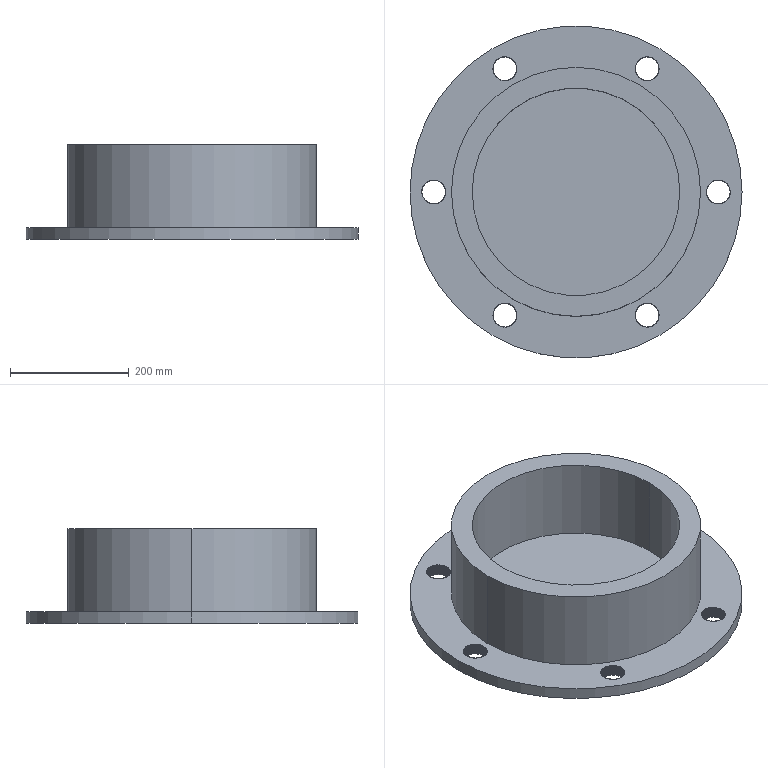Part | SolidWorks | features SweepThread 6, ICE 3, 3DProfileFeature 1, Extrusion 1 | 1 solid | 766 faces | box 560 x 560 x 160 mm | volume 10700722 mm3 | cylinder 732 | spline 18 | plane 16 | commonest cylinder face diameters 40 x726 350 x2 420 x2 560 x2